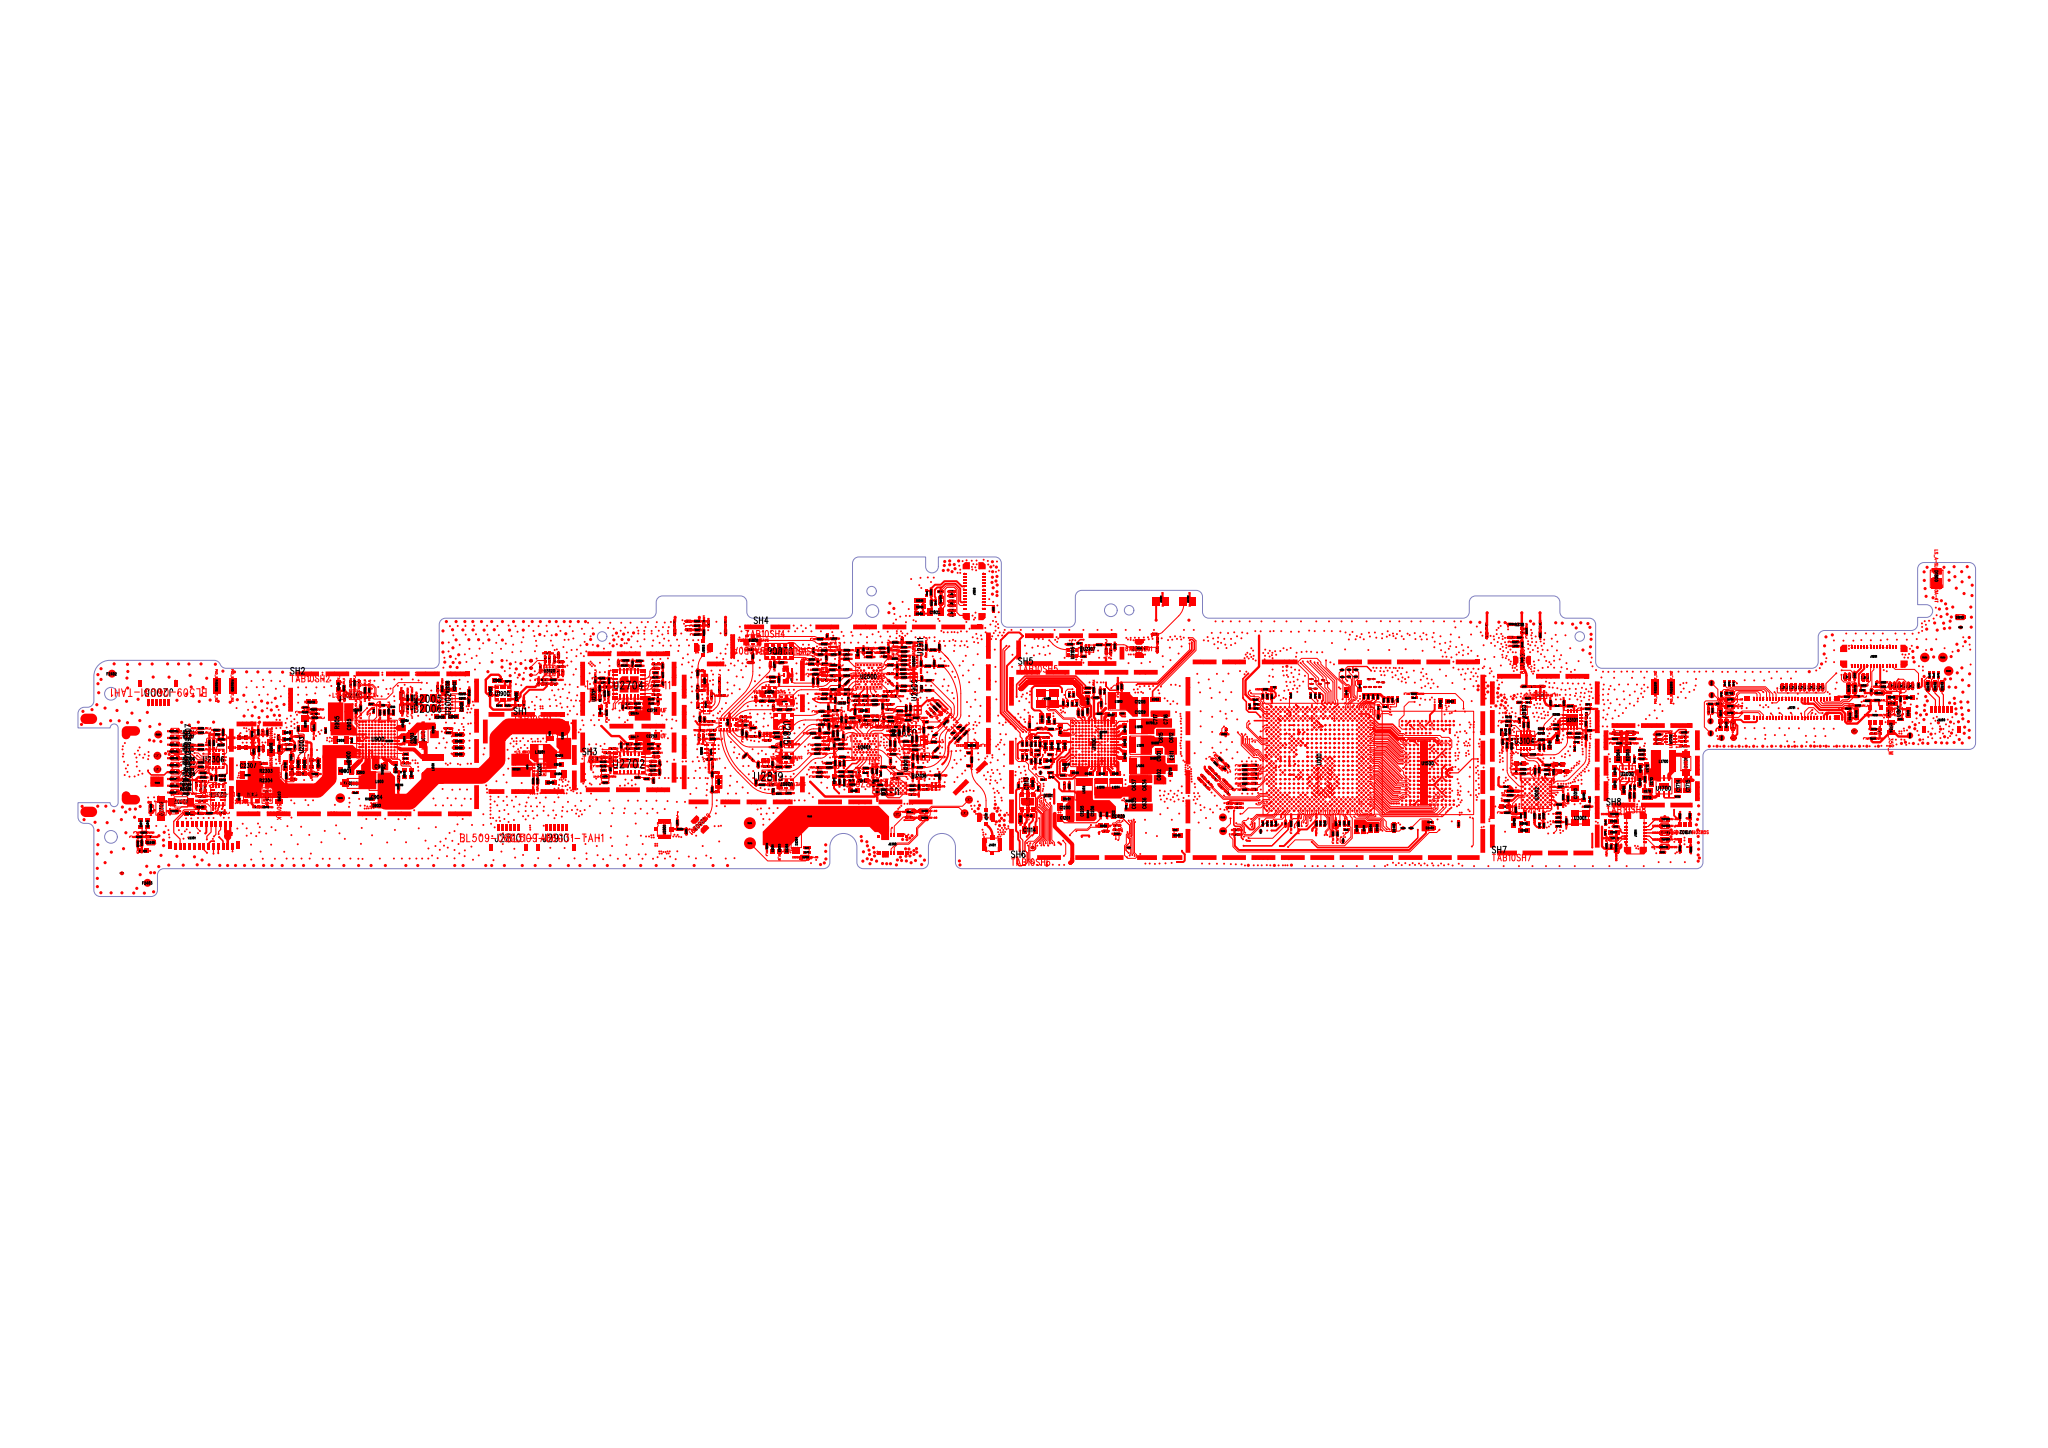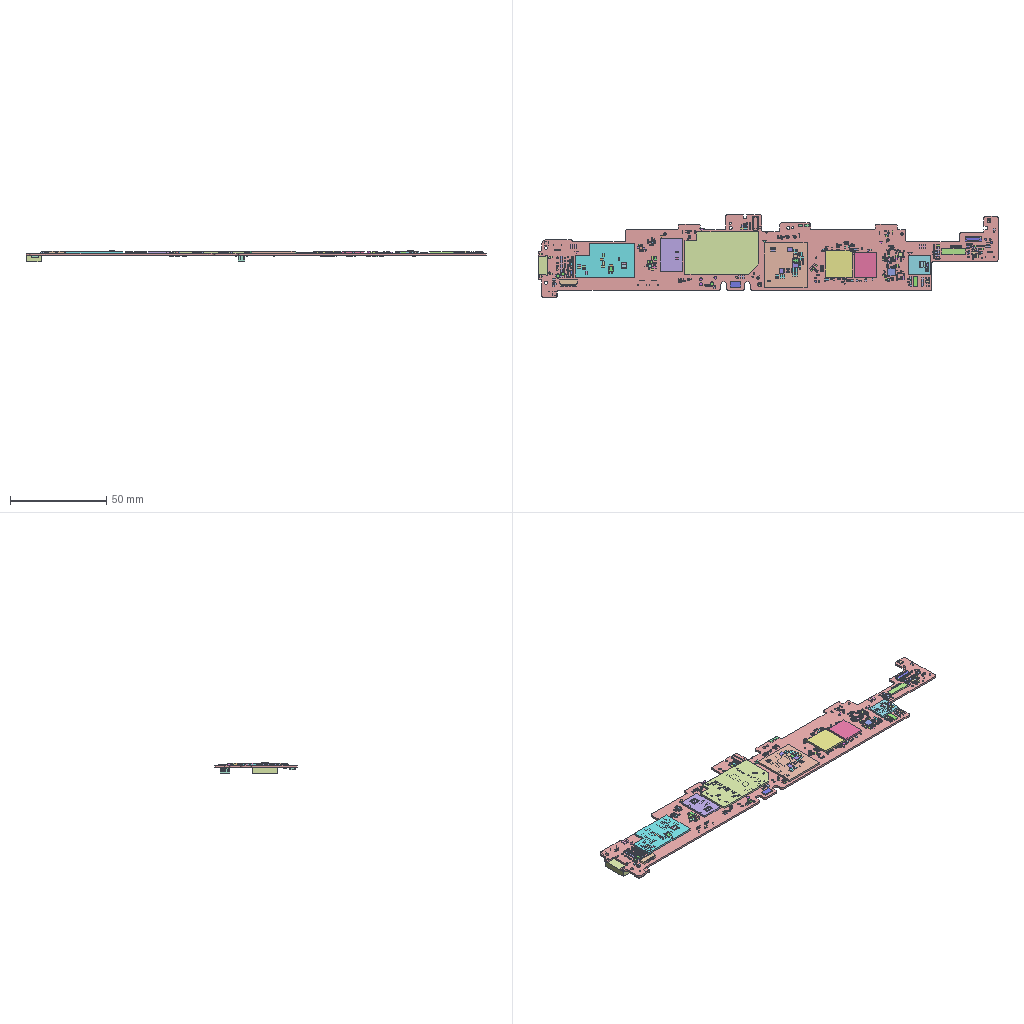Circuit board layout | Siemens PADS | box 238.8 x 42.7 x 5.7 mm
Layer stack:
layer,name,type,plane,layer_thickness_mm,copper_thickness_mm,dielectric_constant
0,,,,0,,3.3
1,Top,ROUTING,NONE,0.1,0.01,4.3
2,Inner Layer 2,ROUTING,NONE,0.1,0.01,4.3
3,Inner Layer 3,ROUTING,NONE,0.1,0.01,4.3
4,Inner Layer 4,ROUTING,NONE,0.1,0.01,4.3
5,Inner Layer 5,ROUTING,NONE,0.1,0.02,4.3
6,Inner Layer 6,ROUTING,NONE,0.1,0.03,4.3
7,Inner Layer 7,ROUTING,NONE,0.254,0.03429,4.3
8,Bottom,ROUTING,NONE,0,0.03,3.3
Part placement, first 449 of 1456 lines:
Ref,PartType,Decal,X_mm,Y_mm,Rotation,Layer,Placed,Installed
ANT2801,LS_4-00-43448,LS_4-00-43448,78.6,32.95,270,Bottom,True,True
ANT2802,LS_4-00-43448,LS_4-00-43448,72,32.95,270,Bottom,True,True
ANT2803,LS_4-00-43448,LS_4-00-43448,75.3,32.95,270,Bottom,True,True
ANT3101,LS_4-00-43448,LS_4-00-43448,132.7,33.65,90,Top,False,True
ANT3103,LS_4-00-43448,LS_4-00-43448,136.1,33.65,90,Top,False,True
ANT3104,LS_4-00-43448,LS_4-00-43448,174.3,32.95,270,Bottom,True,True
ANT3105,LS_4-00-43448,LS_4-00-43448,180.9,32.95,270,Bottom,True,True
ANT3106,LS_4-00-43448,LS_4-00-43448,177.6,32.952,270,Bottom,True,True
B1000,B0402_BLM15AG601SN1D,BEAD0402,37.409,11.935,270,Top,True,True
B1001,B0402_BLM15AG601SN1D,BEAD0402,38.284,11.935,270,Top,True,True
B1401,B0402-BK1005HM102-T,BEAD0402,119.675,15.425,270,Top,True,True
B2000,B0402-BK1005HM102-T,BEAD0402,17.046,16.485,0,Top,True,True
B2001,B0603_BLM18BD252SN1,BEAD0603,20.671,15.185,270,Top,True,True
B2002,B0402-BK1005HM102-T,BEAD0402,17.096,15.26,0,Top,True,True
B2003,B0603_PZ1608U221,BEAD0603,191.3,14.325,90,Top,True,True
B2004,B0603_PZ1608U221,BEAD0603,190.1,14.325,90,Top,True,True
B2005,B0603_PZ1608U221,BEAD0603,40.421,21.46,180,Top,True,True
B2006,B0603_PZ1608U221,BEAD0603,40.421,20.21,180,Top,True,True
B2007,B0402-BLM15HD102SN1,BEAD0402,22.746,16.285,180,Top,True,True
B2008,B0402_BLM15AG601SN1D,BEAD0402,25.721,13.185,270,Top,True,True
B2009,R0402_0R,RES0402_HQ-A,24.871,13.123,270,Top,True,True
B2010,B0402-BK1005HM102-T,BEAD0402,5.1,5.675,270,Top,True,True
B2011,B0402-BK1005HM102-T,BEAD0402,4.25,5.675,270,Top,True,True
B2012,B0603_BLM18BD252SN1,BEAD0603,24.934,18.235,90,Top,True,True
B2013,B0402-BLM15HD102SN1,BEAD0402,22.746,17.135,0,Top,True,True
B2014,R0402_0R,RES0402_HQ-A,24.071,13.123,270,Top,True,True
B3001,B0402_BLM15AG601SN1D,BEAD0402,185.8,9.15,270,Top,True,True
B3002,B0402_BLM15AG601SN1D,BEAD0402,178.3,5.7,0,Top,True,True
C100,C0201_22NF,CAP0201_HQ,154.575,5.725,270,Top,True,True
C101,C0201_100NF_10V_K,CAP0201_HQ,127.15,22.85,270,Top,True,True
C102,C0201_NC,CAP0201_HQ_NC,156.225,5.725,270,Top,True,True
C103,C0201_NC,CAP0201_HQ_NC,155.675,5.725,270,Top,True,True
C104,C0201_100NF_10V_K,CAP0201_HQ,154.225,4.45,270,Top,True,True
C105,C0201_100NF_10V_K,CAP0201_HQ,154.775,4.45,270,Top,True,True
C301,C0201_33PF_25V_J,CAP0201_HQ,146.525,21.7,270,Top,True,True
C302,C0201_33PF_25V_J,CAP0201_HQ,145.7,22.525,0,Top,True,True
C500,C0201_22PF_25V_J,CAP0201_HQ,143.225,10.725,180,Top,True,True
C501,C0201_22PF_25V_J,CAP0201_HQ,143.225,9.975,180,Top,True,True
C502,C0201_22PF_25V_J,CAP0201_HQ,140.15,13.75,135,Top,True,True
C503,C0201_22PF_25V_J,CAP0201_HQ,139.575,13.2,135,Top,True,True
C504,C0201_100NF_10V_K,CAP0201_HQ,148.05,10.825,270,Bottom,True,True
C505,C0201_NC,CAP0201_HQ_NC,138.925,12.525,135,Top,True,True
C506,C0201_NC,CAP0201_HQ_NC,140.697,10.953,135,Top,True,True
C507,C0201_22PF_25V_J,CAP0201_HQ,143.225,12.45,180,Top,True,True
C508,C0201_22PF_25V_J,CAP0201_HQ,143.225,13,180,Top,True,True
C509,C0201_22PF_25V_J,CAP0201_HQ,143.225,11.9,180,Top,True,True
C510,C0201_22PF_25V_J,CAP0201_HQ,143.225,11.35,180,Top,True,True
C511,C0201_NC,CAP0201_HQ_NC,140.122,10.353,315,Top,True,True
C512,C0201_NC,CAP0201_HQ_NC,138.536,12.136,135,Top,True,True
C513,C0201_NC,CAP0201_HQ_NC,141.25,7.7,180,Top,True,True
C514,C0201_NC,CAP0201_HQ_NC,141.25,8.25,180,Top,True,True
C515,C0201_NC,CAP0201_HQ_NC,137.95,11.525,135,Top,True,True
C516,C0201_NC,CAP0201_HQ_NC,137.561,11.136,135,Top,True,True
C600,C0201_100NF_10V_K,CAP0201_HQ,156.125,10.2,270,Bottom,True,True
C601,C0603_22UF_M,CAP0603_L,132.3,14.175,90,Top,True,True
C602,C0603_22UF_M,CAP0603_L,132.3,11.85,270,Top,True,True
C603,C0201_1UF,CAP0201_HQ,153.075,15.55,180,Bottom,True,True
C604,C0201_100NF_10V_K,CAP0201_HQ,151.975,15.55,0,Bottom,True,True
C605,C0201_NC,CAP0201_HQ_NC,157,14.65,180,Bottom,True,True
C606,C0201_NC,CAP0201_HQ_NC,157,14.1,180,Bottom,True,True
C607,C0201_100NF_10V_K,CAP0201_HQ,157,13.55,180,Bottom,True,True
C608,C0201_1UF,CAP0201_HQ,124.987,6.9,270,Top,True,True
C609,C0201_100NF_10V_K,CAP0201_HQ,150.175,9.6,270,Bottom,True,True
C610,C0201_100NF_10V_K,CAP0201_HQ,155.025,17.1,0,Bottom,True,True
C611,C0603_NC,CAP0603_NC,133.9,14.262,270,Top,True,True
C612,C0603_22UF_M,CAP0603_L,133.85,16.525,90,Top,True,True
C613,LS_C0201_1UF_10V_M,CAP0201_HQ,152.725,13.375,90,Bottom,True,True
C614,C0201_100NF_10V_K,CAP0201_HQ,152.325,16.325,180,Bottom,True,True
C615,C0603_22UF_M,CAP0603_L,132.537,16.525,90,Top,True,True
C616,C0201_100NF_10V_K,CAP0201_HQ,153.4,13.175,90,Bottom,True,True
C617,C0201_1UF,CAP0201_HQ,149.3,14.05,0,Bottom,True,True
C618,C0201_100NF_10V_K,CAP0201_HQ,150.4,16.7,90,Bottom,True,True
C619,C0201_100NF_10V_K,CAP0201_HQ,153.65,11.775,0,Bottom,True,True
C620,C0201_2.2UF_6.3V_M,CAP0201_HQ,152.55,11.775,180,Bottom,True,True
C621,C0201_1UF,CAP0201_HQ,151.7,10.425,0,Bottom,True,True
C622,C0402_NC,CAP0402_HQ_NC,126.588,6.9,270,Top,True,True
C623,C0201_1UF,CAP0201_HQ,125.787,6.9,270,Top,True,True
C624,C0201_100NF_10V_K,CAP0201_HQ,157,15.2,180,Bottom,True,True
C625,C0201_100NF_10V_K,CAP0201_HQ,157,12.45,180,Bottom,True,True
C626,C0201_1UF,CAP0201_HQ,152.6,14.525,180,Bottom,True,True
C627,C0201_100NF_10V_K,CAP0201_HQ,150.725,10.125,90,Bottom,True,True
C628,C0201_1UF,CAP0201_HQ,153.475,16.35,180,Bottom,True,True
C629,C0201_100NF_10V_K,CAP0201_HQ,154.5,13.775,90,Bottom,True,True
C630,C0201_100NF_10V_K,CAP0201_HQ,154.15,10.075,0,Bottom,True,True
C631,C0201_2.2UF_6.3V_M,CAP0201_HQ,153.65,11.225,0,Bottom,True,True
C632,C0201_1UF,CAP0201_HQ,151.7,9.875,0,Bottom,True,True
C633,C0201_100NF_10V_K,CAP0201_HQ,154.15,10.625,180,Bottom,True,True
C634,C0603_22UF_M,CAP0603_L,130.475,10.575,90,Top,True,True
C635,C0603_22UF_M,CAP0603_L,129.15,8.275,270,Top,True,True
C636,C0603_22UF_M,CAP0603_L,130.475,8.275,270,Top,True,True
C637,C0603_22UF_M,CAP0603_L,129.15,10.575,90,Top,True,True
C638,LS_C0201_1UF_10V_M,CAP0201_HQ,118.7,17.525,0,Top,True,True
C639,C0201_2.2UF_6.3V_M,CAP0201_HQ,153.675,12.35,180,Bottom,True,True
C640,C0201_100NF_10V_K,CAP0201_HQ,148.8,12.4,0,Bottom,True,True
C641,C0201_1UF,CAP0201_HQ,152.55,11.225,180,Bottom,True,True
C642,C0201_100NF_10V_K,CAP0201_HQ,151.7,9.325,0,Bottom,True,True
C643,C0201_1UF,CAP0201_HQ,154.15,9.525,0,Bottom,True,True
C644,C0201_100NF_10V_K,CAP0201_HQ,151.525,8.5,0,Bottom,True,True
C645,C0201_100NF_10V_K,CAP0201_HQ,155.05,18.875,0,Bottom,True,True
C646,LS_C0201_1UF_10V_M,CAP0201_HQ,156.4,9.375,0,Bottom,True,True
C647,C0201_100NF_10V_K,CAP0201_HQ,150.425,17.975,270,Bottom,True,True
C648,C0201_100NF_10V_K,CAP0201_HQ,148.9,15.9,90,Bottom,True,True
C649,C0201_100NF_10V_K,CAP0201_HQ,148.35,15.9,90,Bottom,True,True
C650,C0201_100NF_10V_K,CAP0201_HQ,149.875,5.675,270,Top,True,True
C651,C0201_100NF_10V_K,CAP0201_HQ,33.025,22.35,90,Top,True,True
C652,C0201_100NF_10V_K,CAP0201_HQ,156.125,17.125,90,Bottom,True,True
C653,C0201_100NF_10V_K,CAP0201_HQ,157,15.75,180,Bottom,True,True
C654,C0201_100NF_10V_K,CAP0201_HQ,148.9,12.95,0,Bottom,True,True
C655,C0201_2.2UF_6.3V_M,CAP0201_HQ,151.85,13.2,0,Bottom,True,True
C700,C0201_1UF,CAP0201_HQ,151.4,17.525,0,Bottom,True,True
C701,C0201_1UF,CAP0201_HQ,151.225,16.975,0,Bottom,True,True
C702,C0201_100NF_10V_K,CAP0201_HQ,153.125,17.575,180,Bottom,True,True
C703,C0201_1UF,CAP0201_HQ,153.075,9.25,90,Bottom,True,True
C704,C0201_100NF_10V_K,CAP0201_HQ,152.125,5.725,270,Top,True,True
C705,C0201_1UF,CAP0201_HQ,151.4,18.075,0,Bottom,True,True
C706,C0201_1UF,CAP0201_HQ,152.7,18.425,180,Bottom,True,True
C707,C0201_1UF,CAP0201_HQ,155.825,12.675,270,Bottom,True,True
C708,C0201_100NF_10V_K,CAP0201_HQ,148.45,13.5,0,Bottom,True,True
C709,C0201_100NF_10V_K,CAP0201_HQ,153.95,13.175,270,Bottom,True,True
C710,C0201_100NF_10V_K,CAP0201_HQ,148,18.175,270,Bottom,True,True
C711,C0201_100NF_10V_K,CAP0201_HQ,148.075,11.85,0,Bottom,True,True
C712,C0201_100NF_10V_K,CAP0201_HQ,151.225,16.425,180,Bottom,True,True
C713,C0201_100NF_10V_K,CAP0201_HQ,147.35,13.5,0,Bottom,True,True
C714,C0201_100NF_10V_K,CAP0201_HQ,147.35,12.95,0,Bottom,True,True
C715,C0201_100NF_10V_K,CAP0201_HQ,147.225,11.1,0,Bottom,True,True
C716,C0603_22UF_M,CAP0603_L,133.15,18.825,90,Top,True,True
C717,C0603_22UF_M,CAP0603_L,131.85,18.825,90,Top,True,True
C718,C0201_100NF_10V_K,CAP0201_HQ,150.75,14.675,180,Bottom,True,True
C719,C0201_100NF_10V_K,CAP0201_HQ,150.75,15.775,180,Bottom,True,True
C720,C0201_1UF,CAP0201_HQ,149.9,10.975,180,Bottom,True,True
C721,C0201_100NF_10V_K,CAP0201_HQ,150.75,14.125,180,Bottom,True,True
C722,C0201_100NF_10V_K,CAP0201_HQ,150.75,13.025,180,Bottom,True,True
C723,C0201_2.2UF_6.3V_M,CAP0201_HQ,155.325,14.05,180,Bottom,True,True
C724,C0201_1UF,CAP0201_HQ,155.475,11.85,180,Bottom,True,True
C725,C0201_2.2UF_6.3V_M,CAP0201_HQ,154.775,12.95,0,Bottom,True,True
C726,C0402_4.7UF_M,CAP0402_L_HQ,133.75,12.3,270,Top,True,True
C727,C0201_2.2UF_6.3V_M,CAP0201_HQ,155.325,13.5,180,Bottom,True,True
C728,C0201_1UF,CAP0201_HQ,154.775,12.4,0,Bottom,True,True
C729,C0201_2.2UF_6.3V_M,CAP0201_HQ,150.75,15.225,180,Bottom,True,True
C730,C0201_1UF,CAP0201_HQ,150.75,13.575,180,Bottom,True,True
C731,C0201_100NF_10V_K,CAP0201_HQ,150.75,12.475,180,Bottom,True,True
C732,C0201_2.2UF_6.3V_M,CAP0201_HQ,150.75,11.925,180,Bottom,True,True
C733,C0201_1UF,CAP0201_HQ,149.9,10.425,180,Bottom,True,True
C734,C0201_100NF_10V_K,CAP0201_HQ,152.775,10.35,90,Bottom,True,True
C735,C0201_100NF_10V_K,CAP0201_HQ,156.15,13.775,270,Bottom,True,True
C736,C0201_2.2UF_6.3V_M,CAP0201_HQ,154.44,14.896,90,Bottom,True,True
C737,C0201_2.2UF_6.3V_M,CAP0201_HQ,154.998,14.881,90,Bottom,True,True
C900,C0603_4.7UF_35V_M,CAP0603,30.344,14.074,270,Top,True,True
C901,C0603_4.7UF_35V_M,CAP0603,30.094,12.34,180,Top,True,True
C902,C0603_4.7UF_10V_K,CAP0603,34.425,12.9,180,Top,True,True
C903,C0402_27NF,CAP0402_HQ,31.975,12.139,0,Top,True,True
C904,C0603_22UF_M,CAP0603_L,33.984,9.047,180,Top,True,True
C905,C0603_NC,CAP0603_NC,30.414,18.186,90,Top,True,True
C906,LS_C0201_1UF_10V_M,CAP0201_HQ,31.896,20.26,270,Top,True,True
C907,LS_C0201_1UF_10V_M,CAP0201_HQ,31.35,19.75,90,Top,True,True
C908,C0603_4.7UF_10V_K,CAP0603,29.425,16.15,180,Top,True,True
C1000,C0201_0.47UF_M,CAP0201_HQ,36.684,11.36,270,Top,True,True
C1001,C0201_100NF_10V_K,CAP0201_HQ,34.321,19.685,270,Top,True,True
C1002,C0201_0.47UF_M,CAP0201_HQ,34.546,20.523,0,Top,True,True
C1003,C0603_4.7UF_35V_M,CAP0603,38.35,16.45,270,Top,True,True
C1004,C0201_18PF,CAP0201_HQ,37.446,16.235,90,Top,True,True
C1005,C0201_100NF_10V_K,CAP0201_HQ,36.684,10.26,90,Top,True,True
C1008,C0402_10UF,CAP0402_L_HQ,37.2,18.225,270,Top,True,True
C1009,C0201_100NF_10V_K,CAP0201_HQ,35.471,19.685,90,Top,True,True
C1012,C0201_NC,CAP0201_HQ_NC,37.596,14.41,0,Top,True,True
C1013,C0402_10UF,CAP0402_L_HQ,36.323,12.764,270,Top,True,True
C1100,C0201_100NF_10V_K,CAP0201_HQ,125.55,16.875,270,Bottom,True,True
C1101,C0201_1UF,CAP0201_HQ,125,16.875,90,Bottom,True,True
C1103,C0201_NC,CAP0201_HQ_NC,119.2,18.475,90,Top,True,True
C1104,C0402_10UF_10V_M,CAP0402_HQ_C,118.475,18.775,90,Top,True,True
C1105,C0201_NC,CAP0201_HQ_NC,127.775,19.525,180,Top,True,True
C1107,C0201_1UF,CAP0201_HQ,122.175,19.625,270,Top,True,True
C1108,C0201_NC,CAP0201_HQ_NC,134.425,4.875,0,Top,True,True
C1109,C0201_1UF,CAP0201_HQ,122.725,19.625,270,Top,True,True
C1110,C0201_NC,CAP0201_HQ_NC,121.45,20.725,90,Top,True,True
C1111,C0201_1NF,CAP0201_HQ,120.35,20.725,90,Top,True,True
C1112,C0201_100NF_10V_K,CAP0201_HQ,116.05,18.075,270,Top,True,True
C1113,C0402_10UF_10V_M,CAP0402_HQ_C,115.625,10.75,90,Top,True,True
C1114,C0603_1UF_50V_K,CAP0603,116.125,4.925,0,Top,True,True
C1115,C0201_NC,CAP0201_HQ_NC,125.625,4.725,180,Top,True,True
C1200,C0603_22UF_M,CAP0603_L,120.575,7.725,180,Top,True,True
C1201,C0603_22UF_M,CAP0603_L,120.575,6.425,180,Top,True,True
C1202,C0402_4.7UF_10V_M,CAP0402_HQ_B,128.037,17.6,90,Top,True,True
C1203,C0402_4.7UF_10V_M,CAP0402_HQ_B,128.037,15.9,90,Top,True,True
C1204,C0402_4.7UF_10V_M,CAP0402_HQ_B,123.487,11.975,0,Top,True,True
C1205,C0603_22UF_M,CAP0603_L,122.638,7.275,270,Top,True,True
C1206,C0603_22UF_M,CAP0603_L,123.938,7.275,270,Top,True,True
C1207,C0402_4.7UF_10V_M,CAP0402_HQ_B,126.362,19.35,180,Top,True,True
C1208,C0603_22UF_M,CAP0603_L,130.025,21.025,0,Top,True,True
C1209,C0603_22UF_M,CAP0603_L,130.025,19.725,0,Top,True,True
C1210,C0402_4.7UF_10V_M,CAP0402_HQ_B,126.888,11.975,0,Top,True,True
C1211,C0402_4.7UF_10V_M,CAP0402_HQ_B,125.188,11.975,0,Top,True,True
C1212,C0402_4.7UF_10V_M,CAP0402_HQ_B,128.037,14.2,90,Top,True,True
C1300,C0201_1UF,CAP0201_HQ,124.95,19.525,180,Top,True,True
C1301,C0402_4.7UF_M,CAP0402_L_HQ,118.525,13.6,0,Top,True,True
C1302,C0201_1UF,CAP0201_HQ,153.325,10.35,90,Bottom,True,True
C1303,C0402_NC,CAP0402_HQ_NC,131.95,21.3,0,Top,True,True
C1304,C0201_100NF_10V_K,CAP0201_HQ,124.175,22.425,90,Top,True,True
C1305,C0201_1UF,CAP0201_HQ,124.4,21.475,0,Top,True,True
C1306,C0402_NC,CAP0402_HQ_NC,117.625,18.85,90,Top,True,True
C1307,C0402_NC,CAP0402_HQ_NC,123.4,21.1,90,Top,True,True
C1308,C0201_NC,CAP0201_HQ_NC,123.35,22.15,0,Top,True,True
C1309,C0402_4.7UF_M,CAP0402_L_HQ,119.925,17.4,90,Top,True,True
C1310,C0201_1UF,CAP0201_HQ,117.375,17.65,180,Top,True,True
C1311,C0201_1UF,CAP0201_HQ,124.95,22.3,270,Top,True,True
C1312,C0201_1UF,CAP0201_HQ,123.4,19.775,90,Top,True,True
C1313,C0201_1UF,CAP0201_HQ,123.35,22.7,0,Top,True,True
C1314,C0201_1UF,CAP0201_HQ,125.125,20.65,90,Top,True,True
C1315,C0201_1UF,CAP0201_HQ,121.05,10.425,270,Top,True,True
C1316,C0201_1UF,CAP0201_HQ,118.225,12.725,0,Top,True,True
C1317,C0201_1UF,CAP0201_HQ,127.7,22.85,90,Top,True,True
C1402,C0201_NC,CAP0201_HQ_NC,117.1,14.875,0,Top,True,True
C1403,C0201_NC,CAP0201_HQ_NC,117.1,14.325,0,Top,True,True
C1404,C0201_NC,CAP0201_HQ_NC,116.3,14.6,270,Top,True,True
C1406,C0201_NC,CAP0201_HQ_NC,115.725,15.7,90,Top,True,True
C1407,C0201_NC,CAP0201_HQ_NC,115.175,15.7,90,Top,True,True
C1408,LS_C0402_2.2UF_10V_M,CAP0402_HQ,120.525,12.825,90,Top,True,True
C1409,LS_C0402_2.2UF_10V_M,CAP0402_HQ,118.85,15.475,90,Top,True,True
C1410,C0402_1UF,CAP0402_HQ,120.5,15.475,270,Top,True,True
C1411,C0201_100NF_6.3V_K,CAP0201_HQ,120.3,11.775,180,Top,True,True
C1412,C0201_1UF,CAP0201_HQ,117.375,15.7,270,Top,True,True
C1413,C0402_2.2UF,CAP0402_HQ,118.05,15.475,270,Top,True,True
C1415,C0201_470PF_K,CAP0201_HQ,116.85,13.5,90,Top,True,True
C1416,C0201_680PF_25V_K,CAP0201_HQ,116.275,15.7,270,Top,True,True
C1417,C0201_680PF_25V_K,CAP0201_HQ,117.05,16.525,180,Top,True,True
C1418,C0201_NC,CAP0201_HQ_NC,115.2,14.05,270,Top,True,True
C1419,C0201_NC,CAP0201_HQ_NC,116.3,13.5,270,Top,True,True
C1420,C0402_2.2UF,CAP0402_HQ,121.85,12.075,180,Top,True,True
C1500,C0201_100NF_10V_K,CAP0201_HQ,164.625,8.225,0,Bottom,True,True
C1501,C0201_100NF_10V_K,CAP0201_HQ,163.6,7.925,90,Bottom,True,True
C1502,C0201_100NF_10V_K,CAP0201_HQ,166.15,17.9,270,Bottom,True,True
C1503,LS_C0201_1UF_10V_M,CAP0201_HQ,164.525,15.95,180,Bottom,True,True
C1504,C0402_NC,CAP0402_HQ_NC,158.975,5.175,270,Top,True,True
C1505,C0402_NC,CAP0402_HQ_NC,159.775,5.175,270,Top,True,True
C1506,C0201_1UF,CAP0201_HQ,163.025,13.65,180,Bottom,True,True
C1507,LS_C0201_1UF_10V_M,CAP0201_HQ,164.6,13.275,180,Bottom,True,True
C1508,C0201_100NF_10V_K,CAP0201_HQ,163.025,13.1,0,Bottom,True,True
C1509,C0201_100NF_10V_K,CAP0201_HQ,163.025,12.55,0,Bottom,True,True
C1510,C0402_4.7UF_M,CAP0402_L_HQ,157.225,5.1,270,Top,True,True
C1511,C0402_4.7UF_M,CAP0402_L_HQ,158.125,5.1,270,Top,True,True
C1512,C0201_1UF,CAP0201_HQ,164.6,12.175,180,Bottom,True,True
C1513,C0201_1UF,CAP0201_HQ,163.175,12,180,Bottom,True,True
C1514,C0201_100NF_10V_K,CAP0201_HQ,164.6,11.625,0,Bottom,True,True
C1515,C0201_100NF_10V_K,CAP0201_HQ,163.175,10.35,0,Bottom,True,True
C1516,C0201_100NF_10V_K,CAP0201_HQ,164.6,9.975,0,Bottom,True,True
C1517,C0201_100NF_10V_K,CAP0201_HQ,164.6,11.075,0,Bottom,True,True
C1518,C0201_100NF_10V_K,CAP0201_HQ,164.6,12.725,0,Bottom,True,True
C1519,LS_C0201_1UF_10V_M,CAP0201_HQ,157,11.9,0,Bottom,True,True
C1520,C0201_1UF,CAP0201_HQ,163.175,11.45,180,Bottom,True,True
C1521,C0201_100NF_10V_K,CAP0201_HQ,163.175,10.9,0,Bottom,True,True
C1522,C0201_100NF_10V_K,CAP0201_HQ,164.6,10.525,0,Bottom,True,True
C1523,C0402_2.2UF,CAP0402_HQ,169.05,21.05,180,Top,True,True
C1524,LS_C0201_1UF_10V_M,CAP0201_HQ,167.3,17.95,180,Bottom,True,True
C1525,C0201_100NF_10V_K,CAP0201_HQ,163.8,17.5,270,Bottom,True,True
C1526,C0201_100NF_10V_K,CAP0201_HQ,167.3,17.4,180,Bottom,True,True
C1527,LS_C0201_1UF_10V_M,CAP0201_HQ,165.475,17.875,270,Bottom,True,True
C1528,C0201_100NF_10V_K,CAP0201_HQ,164.8,17.9,270,Bottom,True,True
C1529,C0201_100NF_10V_K,CAP0201_HQ,164.525,16.5,0,Bottom,True,True
C1530,C0402_1UF,CAP0402_HQ,167.756,20.804,270,Top,True,True
C1531,C0201_100NF_10V_K,CAP0201_HQ,161.775,12.15,0,Bottom,True,True
C1532,C0201_100NF_10V_K,CAP0201_HQ,164.475,22.025,180,Top,True,True
C1700,C0201_100NF_6.3V_K,CAP0201_HQ,222.675,21.15,0,Top,True,True
C1701,C0201_1UF,CAP0201_HQ,195.135,16.838,0,Top,True,True
C1702,C0201_68PF_25V_J,CAP0201_HQ,222.25,16.4,180,Top,True,True
C1703,C0201_1UF,CAP0201_HQ,198.375,17.1,0,Top,True,True
C1704,C0603_4.7UF_35V_M,CAP0603,224.4,17.725,270,Top,True,True
C1706,C0201_39PF_25V_J,CAP0201_HQ,219,21.65,180,Top,True,True
C1707,C0201_39PF_25V_J,CAP0201_HQ,220.25,20.475,0,Top,True,True
C1709,C0201_39PF_25V_J,CAP0201_HQ,219.15,20.175,180,Top,True,True
C1710,C0201_39PF_25V_J,CAP0201_HQ,220.1,21.65,0,Top,True,True
C1711,C0402_1UF,CAP0402_HQ,203.75,18.075,270,Top,True,True
C1712,C0402_NC,CAP0402_HQ_NC,193.757,12.654,90,Top,True,True
C1713,C0402_NC,CAP0402_HQ_NC,194.3,11.025,270,Top,True,True
C1714,C0603_NC,CAP0603_NC,197.65,10.475,270,Top,True,True
C1715,C0603_NC,CAP0603_NC,198.85,10.475,270,Top,True,True
C1716,C0201_NC,CAP0201_HQ_NC,197.625,9.075,0,Top,True,True
C1717,C0201_1UF,CAP0201_HQ,221.575,21.15,180,Top,True,True
C1718,C0201_1UF,CAP0201_HQ,222.25,17.525,0,Top,True,True
C1800,C0201_NC,CAP0201_HQ_NC,104.825,34.85,180,Top,True,True
C1804,C0201_1UF,CAP0201_HQ,103.7,34.675,90,Top,True,True
C1806,C0201_1UF,CAP0201_HQ,103.7,33.475,270,Top,True,True
C1808,C0201_NC,CAP0201_HQ_NC,111.525,32.65,270,Top,True,True
C1809,C0402_10UF,CAP0402_L_HQ,102.225,32.075,0,Top,True,True
C1811,C0402_NC,CAP0402_HQ_NC,226.6,19.6,90,Top,True,True
C1812,C0402_NC,CAP0402_HQ_NC,224.2,19.6,270,Top,True,True
C1815,C0201_1UF,CAP0201_HQ,220.95,23,0,Top,True,True
C1816,C0201_100NF_10V_K,CAP0201_HQ,223.425,22.85,0,Top,True,True
C1817,C0201_1UF,CAP0201_HQ,219.925,24.225,90,Top,True,True
C1818,C0201_1UF,CAP0201_HQ,223.425,23.4,0,Top,True,True
C1819,C0402_10UF,CAP0402_L_HQ,226.75,21.525,0,Top,True,True
C1820,C0201_NC,CAP0201_HQ_NC,221.975,22.275,270,Top,True,True
C1821,C0201_100NF_6.3V_K,CAP0201_HQ,225.625,21.425,270,Top,True,True
C1822,C0603_22UF_M,CAP0603_L,104.225,32.275,0,Top,True,True
C1826,C0201_NC,CAP0201_HQ_NC,227.912,23.062,270,Top,True,True
C1900,C0402_1UF,CAP0402_HQ,51.475,21.675,90,Top,True,True
C1901,C0201_100NF_10V_K,CAP0201_HQ,199.35,3.3,0,Bottom,True,True
C1902,C0402_100NF_16V_K,CAP0402_HQ,49.15,23.7,180,Top,True,True
C1903,C0402_1UF,CAP0402_HQ,48.2,22.325,90,Top,True,True
C1904,C0201_100NF_10V_K,CAP0201_HQ,199.35,2.2,0,Bottom,True,True
C1905,C0201_NC,CAP0201_HQ_NC,197.925,2.475,90,Top,True,True
C1906,C0201_NC,CAP0201_HQ_NC,199.25,2.475,270,Top,True,True
C1907,C0402_2.2UF,CAP0402_HQ,189.6,4.6,180,Top,True,True
C1908,C0402_2.2UF,CAP0402_HQ,189.588,5.987,180,Top,True,True
C1909,C0201_100NF_10V_K,CAP0201_HQ,188.7,2.788,90,Top,True,True
C1910,C0201_NC,CAP0201_HQ_NC,199.175,6.575,90,Top,True,True
C1921,C0201_NC,CAP0201_HQ_NC,111.225,31.95,270,Bottom,True,True
C1922,C0201_1UF,CAP0201_HQ,105.35,33.525,0,Bottom,True,True
C2000,C0402_4.7UF_M,CAP0402_L_HQ,192.9,12.575,90,Top,True,True
C2001,C0201_100NF_10V_K,CAP0201_HQ,193.525,11.175,90,Top,True,True
C2002,LS_C0402_2.2UF_10V_M,CAP0402_HQ,189.7,10.637,270,Top,True,True
C2003,LS_C0402_2.2UF_10V_M,CAP0402_HQ,190.825,9.975,90,Top,True,True
C2006,C0402_4.7UF_10V_M,CAP0402_HQ_B,189.7,12.275,270,Top,True,True
C2007,C0201_100PF_25V_J,CAP0201_HQ,191.425,15.8,180,Top,True,True
C2008,C0201_33PF_25V_J,CAP0201_HQ,192,16.35,180,Top,True,True
C2009,C0201_22NF,CAP0201_HQ,191.625,9.15,90,Top,True,True
C2010,C0201_22NF,CAP0201_HQ,192.175,9.15,90,Top,True,True
C2011,C0201_100PF_25V_J,CAP0201_HQ,190.9,16.35,180,Top,True,True
C2015,C0201_100PF_25V_J,CAP0201_HQ,190.325,15.8,180,Top,True,True
C2016,C0201_33PF_25V_J,CAP0201_HQ,189.8,16.35,180,Top,True,True
C2017,C0201_470PF_K,CAP0201_HQ,22.771,14.985,0,Top,True,True
C2018,C0201_33PF_50V_J,CAP0201_HQ,19.096,15.11,270,Top,True,True
C2019,C0201_33PF_50V_J,CAP0201_HQ,19.071,17.085,90,Top,True,True
C2020,C0201_NC,CAP0201_HQ_NC,19.646,15.11,270,Top,True,True
C2021,C0201_NC,CAP0201_HQ_NC,19.621,17.085,90,Top,True,True
C2022,C0402_4.7UF_M,CAP0402_L_HQ,43.671,22.985,90,Top,True,True
C2023,C0201_100NF_10V_K,CAP0201_HQ,42.146,22.685,270,Top,True,True
C2024,LS_C0402_2.2UF_10V_M,CAP0402_HQ,43.571,19.135,0,Top,True,True
C2025,LS_C0402_2.2UF_10V_M,CAP0402_HQ,44.596,20.385,90,Top,True,True
C2027,C0201_NC,CAP0201_HQ_NC,24.059,17.585,90,Top,True,True
C2028,C0201_33PF_25V_J,CAP0201_HQ,3.85,3.2,270,Top,True,True
C2029,C0201_33PF_50V_J,CAP0201_HQ,26.084,18.96,0,Top,True,True
C2030,C0402_4.7UF_10V_M,CAP0402_HQ_B,41.921,19.085,180,Top,True,True
C2031,C0201_33PF_25V_J,CAP0201_HQ,5.225,4.025,180,Top,True,True
C2032,C0201_33PF_25V_J,CAP0201_HQ,37.796,21.535,270,Top,True,True
C2033,C0201_100PF_25V_J,CAP0201_HQ,4.675,4.575,180,Top,True,True
C2034,C0201_100NF_10V_K,CAP0201_HQ,4.4,3.2,90,Top,True,True
C2035,C0201_100PF_25V_J,CAP0201_HQ,38.896,20.985,270,Top,True,True
C2036,C0201_33PF_25V_J,CAP0201_HQ,4.125,4.025,180,Top,True,True
C2037,C0201_100PF_25V_J,CAP0201_HQ,37.796,20.435,270,Top,True,True
C2038,C0201_33PF_25V_J,CAP0201_HQ,38.346,20.435,270,Top,True,True
C2039,C0201_NC,CAP0201_HQ_NC,21.571,16.46,90,Top,True,True
C2040,C0201_4.7NF_K,CAP0201_HQ,22.584,11.61,90,Top,True,True
C2041,C0402_1NF,CAP0402_HQ_A,24.446,11.947,0,Top,True,True
C2042,C0402_1NF,CAP0402_HQ_A,23.271,12.322,90,Top,True,True
C2043,C0201_NC,CAP0201_HQ_NC,23.421,11.273,0,Top,True,True
C2044,C0402_1UF,CAP0402_HQ,26.559,13.235,90,Top,True,True
C2045,C0201_33PF_50V_J,CAP0201_HQ,24.984,19.71,180,Top,True,True
C2046,C0201_100PF_25V_J,CAP0201_HQ,38.346,21.535,270,Top,True,True
C2047,C0201_22NF,CAP0201_HQ,45.546,21.085,90,Top,True,True
C2048,C0201_22NF,CAP0201_HQ,45.546,22.185,270,Top,True,True
C2049,C0201_33PF_50V_J,CAP0201_HQ,26.084,20.06,180,Top,True,True
C2055,C0201_NC,CAP0201_HQ_NC,57.35,24.625,90,Top,True,True
C2300,C0201_NC,CAP0201_HQ_NC,100.9,6.5,0,Top,True,True
C2301,C0201_NC,CAP0201_HQ_NC,88.075,2.625,180,Top,True,True
C2302,C0201_33PF_25V_J,CAP0201_HQ,83,2.9,270,Top,True,True
C2303,C0402_10UF_10V_M,CAP0402_HQ_C,84.625,2.6,270,Top,True,True
C2304,C0402_10UF_10V_M,CAP0402_HQ_C,83.725,2.6,270,Top,True,True
C2305,C0201_33PF_25V_J,CAP0201_HQ,12.825,6.95,0,Top,True,True
C2306,C0201_33PF_25V_J,CAP0201_HQ,11.725,6.95,0,Top,True,True
C2307,C0603_10UF_25V_M,CAP0603_L,17.8,13.025,180,Top,True,True
C2308,C0603_4.7UF_35V_M,CAP0603,17.7,11.775,0,Top,True,True
C2309,C0402_100NF_50V_M,CAP0402_L_HQ,16.575,9.075,270,Top,True,True
C2310,C0603_1UF_50V_K,CAP0603,21.6,9.1,270,Top,True,True
C2311,C0201_100NF_10V_K,CAP0201_HQ,11.75,12.775,0,Top,True,True
C2312,C0201_100NF_10V_K,CAP0201_HQ,11.75,13.325,0,Top,True,True
C2313,C0201_100NF_10V_K,CAP0201_HQ,11.775,17.625,0,Top,True,True
C2314,C0201_100NF_10V_K,CAP0201_HQ,11.775,17.075,0,Top,True,True
C2315,C0201_NC,CAP0201_HQ_NC,13.134,11.447,270,Top,True,True
C2316,C0201_100NF_10V_K,CAP0201_HQ,13.7,11.45,270,Top,True,True
C2317,C0201_100NF_10V_K,CAP0201_HQ,12.85,15.85,270,Top,True,True
C2318,C0201_100NF_10V_K,CAP0201_HQ,13.4,15.85,270,Top,True,True
C2319,C0201_100NF_10V_K,CAP0201_HQ,11.75,15.525,0,Top,True,True
C2320,C0201_100NF_10V_K,CAP0201_HQ,11.748,14.973,0,Top,True,True
C2321,C0201_100NF_10V_K,CAP0201_HQ,10.05,9.475,180,Top,True,True
C2322,C0201_100NF_10V_K,CAP0201_HQ,10.05,11.175,180,Top,True,True
C2323,C0201_470PF_K,CAP0201_HQ,29.275,21.525,270,Top,True,True
C2324,C0201_470PF_K,CAP0201_HQ,31.175,23.275,90,Top,True,True
C2325,C0201_100NF_10V_K,CAP0201_HQ,148.95,5.7,270,Top,True,True
C2326,LS_C0201_1UF_10V_M,CAP0201_HQ,32.475,22.35,90,Top,True,True
C2327,C0201_100NF_10V_K,CAP0201_HQ,29.825,22.625,90,Top,True,True
C2328,C0402_10UF_10V_M,CAP0402_HQ_C,29.1,22.925,90,Top,True,True
C2355,C0201_100NF_10V_K,CAP0201_HQ,55.1,23.775,180,Top,True,True
C2356,C0201_100NF_10V_K,CAP0201_HQ,56.2,23.775,180,Top,True,True
C2357,C0201_NC,CAP0201_HQ_NC,56.8,26.825,90,Top,True,True
C2358,C0201_NC,CAP0201_HQ_NC,57.075,26,180,Top,True,True
C2400,C0402_10NF_25V,CAP0402_HQ_A,155.925,22.15,270,Top,True,True
C2401,C0402_10NF_25V,CAP0402_HQ_A,157.6,22.975,270,Top,True,True
C2403,C0201_100PF_25V_J,CAP0201_HQ,96.4,10.775,270,Top,True,True
C2501,C0201_1UF,CAP0201_HQ,96.575,20.625,0,Top,True,True
C2502,R0201_51R,RES0201_HQ,96.65,21.725,180,Top,True,True
C2503,C0201_1.2PF_50V_B,CAP0201_HQ,90.275,21.4,180,Top,True,True
C2504,C0201_1UF,CAP0201_HQ,94.1,19.8,270,Top,True,True
C2505,C0201_100NF_6.3V_K,CAP0201_HQ,96.65,21.175,180,Top,True,True
C2506,C0201_10NF,CAP0201_HQ,94.375,21.725,180,Top,True,True
C2507,C0201_0.47UF_M,CAP0201_HQ,94.375,21.175,180,Top,True,True
C2508,C0402_10UF,CAP0402_L_HQ,95.225,19.9,0,Top,True,True
C2509,C0201_1UF,CAP0201_HQ,95.15,27.475,270,Top,True,True
C2510,C0402_10UF,CAP0402_L_HQ,94.425,27.175,270,Top,True,True
C2511,C0201_22PF_25V_J,CAP0201_HQ,97.9,21.725,180,Top,True,True
C2512,C0201_10NF,CAP0201_HQ,95.475,21.725,180,Top,True,True
C2513,C0201_100PF_50V_J,CAP0201_HQ,99,21.725,180,Top,True,True
C2514,C0201_100NF_6.3V_K,CAP0201_HQ,95.475,21.175,180,Top,True,True
C2515,C0201_100NF_6.3V_K,CAP0201_HQ,95.975,27.2,180,Top,True,True
C2516,C0201_10NF,CAP0201_HQ,95.975,26.65,180,Top,True,True
C2517,C0201_1.2PF_25V_C,CAP0201_HQ,90.275,21.95,0,Top,True,True
C2518,C0201_22PF_25V_J,CAP0201_HQ,93.025,21.95,0,Top,True,True
C2519,C0201_22PF_25V_J,CAP0201_HQ,93.025,22.5,0,Top,True,True
C2521,C0201_2.7PF_25V_C,CAP0201_HQ,89.675,12.7,0,Top,True,True
C2522,C0201_2.7PF_25V_C,CAP0201_HQ,89.675,11.6,180,Top,True,True
C2524,C0201_2.7PF_25V_C,CAP0201_HQ,91.65,21.125,90,Top,True,True
C2525,C0201_2.7PF_25V_C,CAP0201_HQ,93.3,21.125,90,Top,True,True
C2552,C0201_33PF_25V_J,CAP0201_HQ,79.925,17.2,270,Top,True,True
C2553,C0201_33PF_25V_J,CAP0201_HQ,80.1,18.025,0,Top,True,True
C2601,C0201_150PF_K,CAP0201_HQ,96.275,12.35,270,Top,True,True
C2602,C0201_150PF_K,CAP0201_HQ,96.825,12.35,270,Top,True,True
C2603,C0402_1UF,CAP0402_HQ,95.125,11.075,0,Top,True,True
C2604,R0201_51R,RES0201_HQ,94.625,12.025,90,Top,True,True
C2605,C0201_22PF_25V_J,CAP0201_HQ,90.825,12.7,0,Top,True,True
C2606,C0201_22PF_25V_J,CAP0201_HQ,92.475,14.025,0,Top,True,True
C2607,R0201_0R,RES0201_HQ,98.45,20.625,0,Top,True,True
C2608,R0201_0R,RES0201_HQ,98.45,20.075,180,Top,True,True
C2609,C0201_150PF_K,CAP0201_HQ,96.625,18.625,0,Top,True,True
C2610,C0201_150PF_K,CAP0201_HQ,97.625,20.35,90,Top,True,True
C2611,C0201_1UF,CAP0201_HQ,92.2,10.825,90,Top,True,True
C2612,C0201_0.47UF_M,CAP0201_HQ,92.475,11.65,180,Top,True,True
C2613,C0201_10NF,CAP0201_HQ,92.475,12.2,180,Top,True,True
C2614,C0201_100NF_6.3V_K,CAP0201_HQ,95.45,12.625,0,Top,True,True
C2615,C0201_2PF,CAP0201_HQ,92.75,13.2,90,Top,True,True
C2616,C0201_2.2PF_50V_C,CAP0201_HQ,91.65,13.2,90,Top,True,True
C2617,C0402_10UF,CAP0402_L_HQ,91.475,11.125,90,Top,True,True
C2618,C0402_10UF,CAP0402_L_HQ,94,9.825,0,Top,True,True
C2619,C0201_1UF,CAP0201_HQ,93.7,10.55,0,Top,True,True
C2620,C0201_100NF_6.3V_K,CAP0201_HQ,93.6,11.65,180,Top,True,True
C2621,C0201_10NF,CAP0201_HQ,93.6,12.2,180,Top,True,True
C2622,C0201_100NF_6.3V_K,CAP0201_HQ,95.525,19.175,0,Top,True,True
C2623,C0201_10NF,CAP0201_HQ,95.525,18.625,0,Top,True,True
C2624,C0201_100PF_50V_J,CAP0201_HQ,96.675,11.05,0,Top,True,True
C2625,C0201_22PF_25V_J,CAP0201_HQ,97.65,12.775,0,Top,True,True
C2626,R0201_0R,RES0201_HQ,96.625,19.2,0,Top,True,True
C2627,R0201_0R,RES0201_HQ,95.55,18.075,0,Top,True,True
C2703,C0201_NC,CAP0201_HQ_NC,66.775,11.475,0,Top,True,True
C2704,C0201_100PF_25V_J,CAP0201_HQ,66.825,15.15,180,Top,True,True
C2705,C0201_0.47UF_M,CAP0201_HQ,66.825,15.7,180,Top,True,True
C2706,C0201_NC,CAP0201_HQ_NC,68.7,11.85,180,Top,True,True
C2707,C0201_100PF_25V_J,CAP0201_HQ,68.45,15.15,180,Top,True,True
C2708,C0201_100NF_10V_K,CAP0201_HQ,68.45,15.7,180,Top,True,True
C2709,C0201_NC,CAP0201_HQ_NC,68.7,13.5,180,Top,True,True
C2710,C0201_100PF_25V_J,CAP0201_HQ,65.7,15.7,180,Top,True,True
Pad and via stacks:
via_name,drill_mm,start_layer,end_layer,type,pad_size_top,pad_size_inner,pad_size_bottom
JMPVIA_AAAAA,0.9398,1,8,through,1.397,1.778,1.397
VIA1-2,0.1,1,2,micro (1 layer span),0.25,0.25,0.25
VIA2-3,0.1,2,3,buried,0.25,0.25,0.25
VIA1-3,0.1,1,3,blind/micro,0.25,0.25,0.25
VIA6-7,0.1,6,7,buried,0.25,0.25,0.25
VIA7-8,0.1,7,8,micro (1 layer span),0.25,0.25,0.25
VIA6-8,0.1,6,8,blind/micro,0.25,0.25,0.25
VIA1-8,0.2,1,8,through,0.4,0.4,0.4
VIA3-6A,0.2,3,6,buried,0.4,0.4,0.4
Design rules, without the lines most boards share, first 365 of 27833 lines:
# PADS Layout design rules of , as PADS writes them (units: mm)
THERLINEWID 0.381
THERSMDWID 0.254
THERFLAGS 1044735
HATCHGRID 0.1
MINHATAREA 0
HATCHMODE 0
DRILLHOLE 0.1524
DRLOVERSIZE 0
VIAMODE A
LAYERPAIR 3      6
TEARDROP 2713690
RULES_SECTION METRIC
{
NET_CLASS DATA
{
NET_CLASS 100OM
NET_CLASS IQ
NET_CLASS 90OM
NET_CLASS 50OM
NET_CLASS 50OM_2
}
GROUP DATA
ASSOCIATED_NET DATA
DESIGN RULES
{
RULE_SET (1)
{
FOR :
{
DEFAULT :
}
AGAINST :
{
DEFAULT :
}
LAYER 0
CLEARANCE_RULE :
{
TRACK_TO_TRACK 0.075
VIA_TO_TRACK 0.075
VIA_TO_VIA 0.075
PAD_TO_TRACK 0.075
PAD_TO_VIA 0.075
PAD_TO_PAD 0.075
SMD_TO_TRACK 0.075
SMD_TO_VIA 0.075
SMD_TO_PAD 0.075
SMD_TO_SMD 0.075
COPPER_TO_TRACK 0.1
COPPER_TO_VIA 0.1
COPPER_TO_PAD 0.1
COPPER_TO_SMD 0.1
COPPER_TO_COPPER 0.1
TEXT_TO_TRACK 0.1
TEXT_TO_VIA 0.1
TEXT_TO_PAD 0.1
TEXT_TO_SMD 0.1
OUTLINE_TO_TRACK 0.2
OUTLINE_TO_VIA 0.2
OUTLINE_TO_PAD 0.2
OUTLINE_TO_SMD 0.2
OUTLINE_TO_COPPER 0.2
DRILL_TO_TRACK 0.15
DRILL_TO_VIA 0
DRILL_TO_PAD 0.15
DRILL_TO_SMD 0.15
DRILL_TO_COPPER 0.15
SAME_NET_SMD_TO_VIA 0
SAME_NET_SMD_TO_CRN 0
SAME_NET_VIA_TO_VIA 0
SAME_NET_PAD_TO_CRN 0
MIN_TRACK_WIDTH 0.05
REC_TRACK_WIDTH 0.075
MAX_TRACK_WIDTH 6
DRILL_TO_DRILL 0
BODY_TO_BODY 0.15
SAME_NET_TRACK_TO_CRN 0
}
}
RULE_SET (2)
{
FOR :
{
NET_CLASS 100OM
}
AGAINST :
{
DEFAULT :
}
LAYER 0
CLEARANCE_RULE :
{
TRACK_TO_TRACK 0.15
VIA_TO_TRACK 0.15
VIA_TO_VIA 0.15
PAD_TO_TRACK 0.1
PAD_TO_VIA 0.1
PAD_TO_PAD 0.1
SMD_TO_TRACK 0.1
SMD_TO_VIA 0.1
SMD_TO_PAD 0.1
SMD_TO_SMD 0.1
COPPER_TO_TRACK 0.15
COPPER_TO_VIA 0.15
COPPER_TO_PAD 0.15
COPPER_TO_SMD 0.15
COPPER_TO_COPPER 0.15
TEXT_TO_TRACK 0.1
TEXT_TO_VIA 0.1
TEXT_TO_PAD 0.1
TEXT_TO_SMD 0.1
OUTLINE_TO_TRACK 0.2
OUTLINE_TO_VIA 0.2
OUTLINE_TO_PAD 0.2
OUTLINE_TO_SMD 0.2
OUTLINE_TO_COPPER 0.2
DRILL_TO_TRACK 0.15
DRILL_TO_VIA 0
DRILL_TO_PAD 0.15
DRILL_TO_SMD 0.15
DRILL_TO_COPPER 0.15
SAME_NET_SMD_TO_VIA 0
SAME_NET_SMD_TO_CRN 0
SAME_NET_VIA_TO_VIA 0
SAME_NET_PAD_TO_CRN 0
MIN_TRACK_WIDTH 0.05
REC_TRACK_WIDTH 0.075
MAX_TRACK_WIDTH 6
DRILL_TO_DRILL 0.15
BODY_TO_BODY 0.15
SAME_NET_TRACK_TO_CRN 0
}
}
RULE_SET (3)
{
FOR :
{
NET_CLASS 90OM
}
AGAINST :
{
DEFAULT :
}
LAYER 0
CLEARANCE_RULE :
{
TRACK_TO_TRACK 0.15
VIA_TO_TRACK 0.15
VIA_TO_VIA 0.15
PAD_TO_TRACK 0.1
PAD_TO_VIA 0.1
PAD_TO_PAD 0.1
SMD_TO_TRACK 0.1
SMD_TO_VIA 0.1
SMD_TO_PAD 0.1
SMD_TO_SMD 0.1
COPPER_TO_TRACK 0.15
COPPER_TO_VIA 0.15
COPPER_TO_PAD 0.15
COPPER_TO_SMD 0.15
COPPER_TO_COPPER 0.15
TEXT_TO_TRACK 0.1
TEXT_TO_VIA 0.1
TEXT_TO_PAD 0.1
TEXT_TO_SMD 0.1
OUTLINE_TO_TRACK 0.2
OUTLINE_TO_VIA 0.2
OUTLINE_TO_PAD 0.2
OUTLINE_TO_SMD 0.2
OUTLINE_TO_COPPER 0.2
DRILL_TO_TRACK 0.15
DRILL_TO_VIA 0
DRILL_TO_PAD 0.15
DRILL_TO_SMD 0.15
DRILL_TO_COPPER 0.15
SAME_NET_SMD_TO_VIA 0
SAME_NET_SMD_TO_CRN 0
SAME_NET_VIA_TO_VIA 0
SAME_NET_PAD_TO_CRN 0
MIN_TRACK_WIDTH 0.05
REC_TRACK_WIDTH 0.075
MAX_TRACK_WIDTH 6
DRILL_TO_DRILL 0.15
BODY_TO_BODY 0.15
SAME_NET_TRACK_TO_CRN 0
}
}
RULE_SET (4)
{
FOR :
{
NET_CLASS 50OM
}
AGAINST :
{
DEFAULT :
}
LAYER 0
CLEARANCE_RULE :
{
TRACK_TO_TRACK 0.2
VIA_TO_TRACK 0.2
VIA_TO_VIA 0.2
PAD_TO_TRACK 0.1
PAD_TO_VIA 0.1
PAD_TO_PAD 0.1
SMD_TO_TRACK 0.1
SMD_TO_VIA 0.1
SMD_TO_PAD 0.1
SMD_TO_SMD 0.1
COPPER_TO_TRACK 0.2
COPPER_TO_VIA 0.2
COPPER_TO_PAD 0.2
COPPER_TO_SMD 0.2
COPPER_TO_COPPER 0.2
TEXT_TO_TRACK 0.1
TEXT_TO_VIA 0.1
TEXT_TO_PAD 0.1
TEXT_TO_SMD 0.1
OUTLINE_TO_TRACK 0.2
OUTLINE_TO_VIA 0.2
OUTLINE_TO_PAD 0.2
OUTLINE_TO_SMD 0.2
OUTLINE_TO_COPPER 0.2
DRILL_TO_TRACK 0.15
DRILL_TO_VIA 0
DRILL_TO_PAD 0.15
DRILL_TO_SMD 0.15
DRILL_TO_COPPER 0.15
SAME_NET_SMD_TO_VIA 0
SAME_NET_SMD_TO_CRN 0
SAME_NET_VIA_TO_VIA 0
SAME_NET_PAD_TO_CRN 0
MIN_TRACK_WIDTH 0.05
REC_TRACK_WIDTH 0.1
MAX_TRACK_WIDTH 6
DRILL_TO_DRILL 0.15
BODY_TO_BODY 0.15
SAME_NET_TRACK_TO_CRN 0
}
}
RULE_SET (5)
{
FOR :
{
NET_CLASS 50OM_2
}
AGAINST :
{
DEFAULT :
}
LAYER 0
CLEARANCE_RULE :
{
TRACK_TO_TRACK 0.075
VIA_TO_TRACK 0.075
VIA_TO_VIA 0.075
PAD_TO_TRACK 0.075
PAD_TO_VIA 0.075
PAD_TO_PAD 0.075
SMD_TO_TRACK 0.075
SMD_TO_VIA 0.075
SMD_TO_PAD 0.075
SMD_TO_SMD 0.075
COPPER_TO_TRACK 0.3
COPPER_TO_VIA 0.3
COPPER_TO_PAD 0.3
COPPER_TO_SMD 0.3
COPPER_TO_COPPER 0.3
TEXT_TO_TRACK 0.1
TEXT_TO_VIA 0.1
TEXT_TO_PAD 0.1
TEXT_TO_SMD 0.1
OUTLINE_TO_TRACK 0.2
OUTLINE_TO_VIA 0.2
OUTLINE_TO_PAD 0.2
OUTLINE_TO_SMD 0.2
OUTLINE_TO_COPPER 0.2
DRILL_TO_TRACK 0.15
DRILL_TO_VIA 0
DRILL_TO_PAD 0.15
DRILL_TO_SMD 0.15
DRILL_TO_COPPER 0.15
SAME_NET_SMD_TO_VIA 0
SAME_NET_SMD_TO_CRN 0
SAME_NET_VIA_TO_VIA 0
SAME_NET_PAD_TO_CRN 0
MIN_TRACK_WIDTH 0.05
REC_TRACK_WIDTH 0.075
MAX_TRACK_WIDTH 6
DRILL_TO_DRILL 0.15
BODY_TO_BODY 0.15
SAME_NET_TRACK_TO_CRN 0
}
}
RULE_SET (6)
{
FOR :
{
NET MIPI_DSI0_LANE1_N
}
AGAINST :
{
DEFAULT :
}
LAYER 0
CLEARANCE_RULE :
{
TRACK_TO_TRACK 0.15
VIA_TO_TRACK 0.1
VIA_TO_VIA 0.1
PAD_TO_TRACK 0.075
PAD_TO_VIA 0.075
PAD_TO_PAD 0.075
SMD_TO_TRACK 0.075
SMD_TO_VIA 0.075
SMD_TO_PAD 0.075
SMD_TO_SMD 0.075
COPPER_TO_TRACK 0.15
COPPER_TO_VIA 0.15
COPPER_TO_PAD 0.15
COPPER_TO_SMD 0.15
COPPER_TO_COPPER 0.15
TEXT_TO_TRACK 0.1
TEXT_TO_VIA 0.1
TEXT_TO_PAD 0.1
TEXT_TO_SMD 0.1
OUTLINE_TO_TRACK 0.2
OUTLINE_TO_VIA 0.2
OUTLINE_TO_PAD 0.2
OUTLINE_TO_SMD 0.2
OUTLINE_TO_COPPER 0.2
DRILL_TO_TRACK 0.15
DRILL_TO_VIA 0
DRILL_TO_PAD 0.15
DRILL_TO_SMD 0.15
DRILL_TO_COPPER 0.15
SAME_NET_SMD_TO_VIA 0
SAME_NET_SMD_TO_CRN 0
SAME_NET_VIA_TO_VIA 0
SAME_NET_PAD_TO_CRN 0
MIN_TRACK_WIDTH 0.05
REC_TRACK_WIDTH 0.09
MAX_TRACK_WIDTH 6
DRILL_TO_DRILL 0
BODY_TO_BODY 0.15
SAME_NET_TRACK_TO_CRN 0
}
}
RULE_SET (7)
{
FOR :
{
NET MIPI_DSI0_LANE1_P
}
AGAINST :
{
DEFAULT :
}
LAYER 0
CLEARANCE_RULE :
{
TRACK_TO_TRACK 0.15
VIA_TO_TRACK 0.1
Classes set for this board:
# PADS net classes of 
NET_CLASS DATA
{
NET_CLASS 100OM
NET_CLASS IQ
NET_CLASS 90OM
NET_CLASS 50OM
NET_CLASS 50OM_2
}